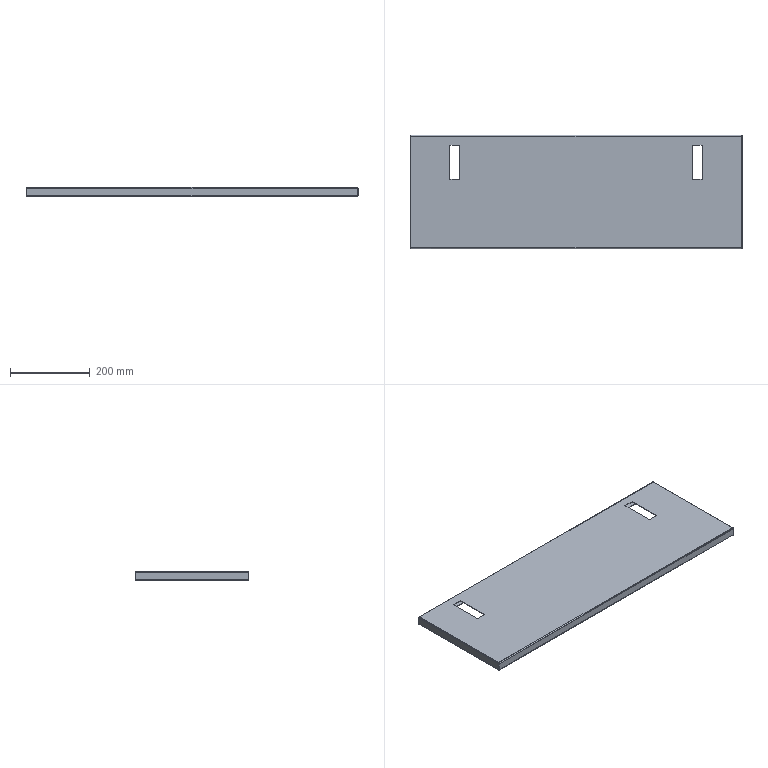Part | SolidWorks | features EdgeFlange 2, FlatPattern 1, ICE 1, MirrorPattern 1, SMBaseFlange 1, SheetMetal 1 | 1 solid | 78 faces | box 834 x 286 x 23 mm | volume 462099 mm3 | plane 46 | spline 16 | cylinder 16 | commonest cylinder face diameters 2 x8 5 x8